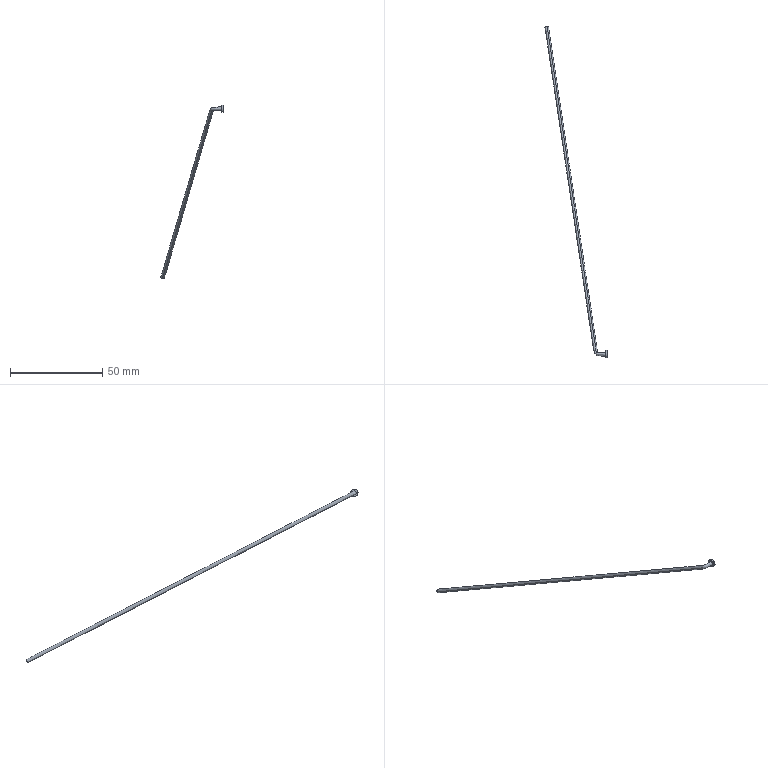Part | STEP file | BREP_70 | 1 solid | 7 faces | box 33.776 x 180.404 x 94.376 mm | volume 676.26 mm3 | plane 3 | cylinder 2 | spline 2 | commonest cylinder face diameters 4 x2